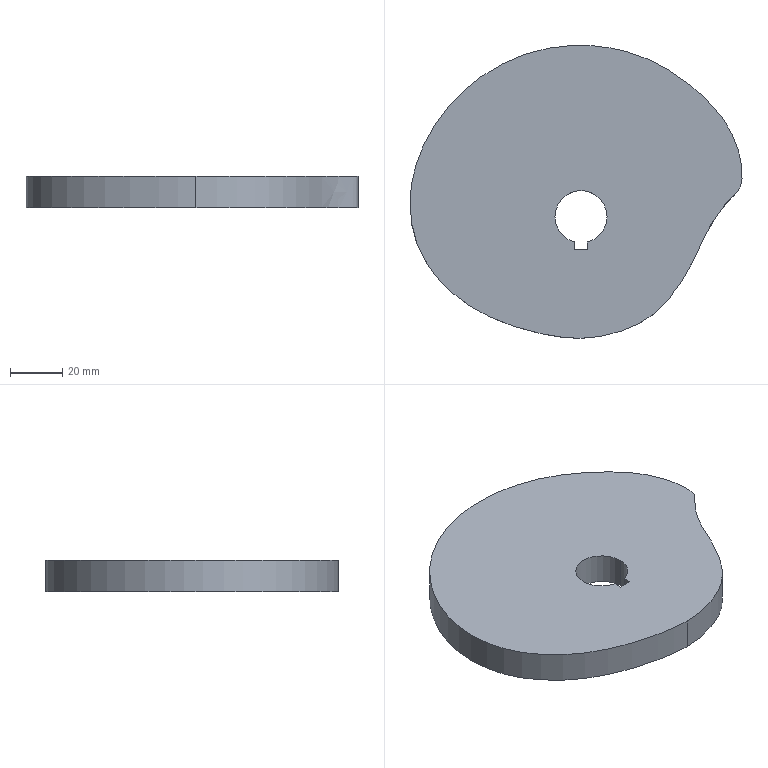Part | SolidWorks | features Extrusion 1 | 1 solid | 10 faces | box 127.495 x 112.48 x 12 mm | volume 126053 mm3 | plane 5 | cylinder 3 | spline 2 | commonest cylinder face diameters 20 x3
STEP:
#1=CARTESIAN_POINT('',(104.838,4.832,12.));
#2=VERTEX_POINT('',#1);
#3=CARTESIAN_POINT('',(99.807,-107.454,12.));
#4=VERTEX_POINT('',#3);
#5=CARTESIAN_POINT('',(104.838,4.832,12.));
#6=CARTESIAN_POINT('',(100.163,5.182,12.));
#7=CARTESIAN_POINT('',(90.7,4.929,12.));
#8=CARTESIAN_POINT('',(77.361,1.638,12.));
#9=CARTESIAN_POINT('',(64.795,-4.533,12.));
#10=CARTESIAN_POINT('',(55.618,-11.622,12.));
#11=CARTESIAN_POINT('',(49.26,-18.351,12.));
#12=CARTESIAN_POINT('',(43.576,-25.792,12.));
#13=CARTESIAN_POINT('',(39.125,-34.043,12.));
#14=CARTESIAN_POINT('',(36.234,-42.572,12.));
#15=CARTESIAN_POINT('',(34.893,-48.983,12.));
#16=CARTESIAN_POINT('',(34.421,-55.273,12.));
#17=CARTESIAN_POINT('',(34.796,-61.595,12.));
#18=CARTESIAN_POINT('',(35.964,-67.585,12.));
#19=CARTESIAN_POINT('',(37.777,-72.838,12.));
#20=CARTESIAN_POINT('',(40.255,-77.705,12.));
#21=CARTESIAN_POINT('',(43.305,-82.213,12.));
#22=CARTESIAN_POINT('',(46.799,-86.338,12.));
#23=CARTESIAN_POINT('',(51.787,-91.146,12.));
#24=CARTESIAN_POINT('',(58.741,-96.133,12.));
#25=CARTESIAN_POINT('',(66.65,-100.026,12.));
#26=CARTESIAN_POINT('',(73.439,-102.579,12.));
#27=CARTESIAN_POINT('',(78.673,-104.2,12.));
#28=CARTESIAN_POINT('',(84.12,-105.561,12.));
#29=CARTESIAN_POINT('',(89.642,-106.65,12.));
#30=CARTESIAN_POINT('',(94.019,-107.214,12.));
#31=CARTESIAN_POINT('',(97.386,-107.433,12.));
#32=CARTESIAN_POINT('',(99.005,-107.461,12.));
#33=CARTESIAN_POINT('',(99.807,-107.454,12.));
#34=B_SPLINE_CURVE_WITH_KNOTS('',3,(#5,#6,#7,#8,#9,#10,#11,#12,#13,#14,#15,#16,#17,#18,#19,#20,#21,#22,#23,#24,#25,#26,#27,#28,#29,#30,#31,#32,#33),.UNSPECIFIED.,.F.,.F.,(4,1,1,1,1,1,1,1,1,1,1,1,1,1,1,1,1,1,1,1,1,1,1,1,1,1,4),(1.5,1.531,1.562,1.594,1.625,1.641,1.656,1.687,1.703,1.719,1.734,1.75,1.766,1.781,1.797,1.812,1.828,1.844,1.875,1.906,1.922,1.937,1.953,1.969,1.984,1.992,2.),.UNSPECIFIED.);
#35=EDGE_CURVE('',#2,#4,#34,.T.);
#36=ORIENTED_EDGE('',*,*,#35,.F.);
#37=CARTESIAN_POINT('',(104.838,4.832,0.));
#38=VERTEX_POINT('',#37);
#39=CARTESIAN_POINT('',(104.838,4.832,12.));
#40=DIRECTION('',(0.,0.,-1.));
#41=VECTOR('',#40,1000.);
#42=LINE('',#39,#41);
#43=EDGE_CURVE('',#2,#38,#42,.T.);
#44=ORIENTED_EDGE('',*,*,#43,.T.);
#45=CARTESIAN_POINT('',(99.807,-107.454,0.));
#46=VERTEX_POINT('',#45);
#47=CARTESIAN_POINT('',(104.838,4.832,0.));
#48=CARTESIAN_POINT('',(100.163,5.182,0.));
#49=CARTESIAN_POINT('',(90.7,4.929,0.));
#50=CARTESIAN_POINT('',(77.361,1.638,0.));
#51=CARTESIAN_POINT('',(64.795,-4.533,0.));
#52=CARTESIAN_POINT('',(55.618,-11.622,0.));
#53=CARTESIAN_POINT('',(49.26,-18.351,0.));
#54=CARTESIAN_POINT('',(43.576,-25.792,0.));
#55=CARTESIAN_POINT('',(39.125,-34.043,0.));
#56=CARTESIAN_POINT('',(36.234,-42.572,0.));
#57=CARTESIAN_POINT('',(34.893,-48.983,0.));
#58=CARTESIAN_POINT('',(34.421,-55.273,0.));
#59=CARTESIAN_POINT('',(34.796,-61.595,0.));
#60=CARTESIAN_POINT('',(35.964,-67.585,0.));
#61=CARTESIAN_POINT('',(37.777,-72.838,0.));
#62=CARTESIAN_POINT('',(40.255,-77.705,0.));
#63=CARTESIAN_POINT('',(43.305,-82.213,0.));
#64=CARTESIAN_POINT('',(46.799,-86.338,0.));
#65=CARTESIAN_POINT('',(51.787,-91.146,0.));
#66=CARTESIAN_POINT('',(58.741,-96.133,0.));
#67=CARTESIAN_POINT('',(66.65,-100.026,0.));
#68=CARTESIAN_POINT('',(73.439,-102.579,0.));
#69=CARTESIAN_POINT('',(78.673,-104.2,0.));
#70=CARTESIAN_POINT('',(84.12,-105.561,0.));
#71=CARTESIAN_POINT('',(89.642,-106.65,0.));
#72=CARTESIAN_POINT('',(94.019,-107.214,0.));
#73=CARTESIAN_POINT('',(97.386,-107.433,0.));
#74=CARTESIAN_POINT('',(99.005,-107.461,0.));
#75=CARTESIAN_POINT('',(99.807,-107.454,0.));
#76=B_SPLINE_CURVE_WITH_KNOTS('',3,(#47,#48,#49,#50,#51,#52,#53,#54,#55,#56,#57,#58,#59,#60,#61,#62,#63,#64,#65,#66,#67,#68,#69,#70,#71,#72,#73,#74,#75),.UNSPECIFIED.,.F.,.F.,(4,1,1,1,1,1,1,1,1,1,1,1,1,1,1,1,1,1,1,1,1,1,1,1,1,1,4),(1.5,1.531,1.562,1.594,1.625,1.641,1.656,1.687,1.703,1.719,1.734,1.75,1.766,1.781,1.797,1.812,1.828,1.844,1.875,1.906,1.922,1.937,1.953,1.969,1.984,1.992,2.),.UNSPECIFIED.);
#77=EDGE_CURVE('',#38,#46,#76,.T.);
#78=ORIENTED_EDGE('',*,*,#77,.T.);
#79=CARTESIAN_POINT('',(99.807,-107.454,12.));
#80=DIRECTION('',(0.,0.,-1.));
#81=VECTOR('',#80,1000.);
#82=LINE('',#79,#81);
#83=EDGE_CURVE('',#4,#46,#82,.T.);
#84=ORIENTED_EDGE('',*,*,#83,.F.);
#85=EDGE_LOOP('',(#36,#44,#78,#84));
#86=FACE_OUTER_BOUND('',#85,.T.);
#87=CARTESIAN_POINT('',(104.838,4.832,12.));
#88=CARTESIAN_POINT('',(104.838,4.832,0.));
#89=CARTESIAN_POINT('',(100.163,5.182,12.));
#90=CARTESIAN_POINT('',(100.163,5.182,0.));
#91=CARTESIAN_POINT('',(90.7,4.929,12.));
#92=CARTESIAN_POINT('',(90.7,4.929,0.));
#93=CARTESIAN_POINT('',(77.361,1.638,12.));
#94=CARTESIAN_POINT('',(77.361,1.638,0.));
#95=CARTESIAN_POINT('',(64.795,-4.533,12.));
#96=CARTESIAN_POINT('',(64.795,-4.533,0.));
#97=CARTESIAN_POINT('',(55.618,-11.622,12.));
#98=CARTESIAN_POINT('',(55.618,-11.622,0.));
#99=CARTESIAN_POINT('',(49.26,-18.351,12.));
#100=CARTESIAN_POINT('',(49.26,-18.351,0.));
#101=CARTESIAN_POINT('',(43.576,-25.792,12.));
#102=CARTESIAN_POINT('',(43.576,-25.792,0.));
#103=CARTESIAN_POINT('',(39.125,-34.043,12.));
#104=CARTESIAN_POINT('',(39.125,-34.043,0.));
#105=CARTESIAN_POINT('',(36.234,-42.572,12.));
#106=CARTESIAN_POINT('',(36.234,-42.572,0.));
#107=CARTESIAN_POINT('',(34.893,-48.983,12.));
#108=CARTESIAN_POINT('',(34.893,-48.983,0.));
#109=CARTESIAN_POINT('',(34.421,-55.273,12.));
#110=CARTESIAN_POINT('',(34.421,-55.273,0.));
#111=CARTESIAN_POINT('',(34.796,-61.595,12.));
#112=CARTESIAN_POINT('',(34.796,-61.595,0.));
#113=CARTESIAN_POINT('',(35.964,-67.585,12.));
#114=CARTESIAN_POINT('',(35.964,-67.585,0.));
#115=CARTESIAN_POINT('',(37.777,-72.838,12.));
#116=CARTESIAN_POINT('',(37.777,-72.838,0.));
#117=CARTESIAN_POINT('',(40.255,-77.705,12.));
#118=CARTESIAN_POINT('',(40.255,-77.705,0.));
#119=CARTESIAN_POINT('',(43.305,-82.213,12.));
#120=CARTESIAN_POINT('',(43.305,-82.213,0.));
#121=CARTESIAN_POINT('',(46.799,-86.338,12.));
#122=CARTESIAN_POINT('',(46.799,-86.338,0.));
#123=CARTESIAN_POINT('',(51.787,-91.146,12.));
#124=CARTESIAN_POINT('',(51.787,-91.146,0.));
#125=CARTESIAN_POINT('',(58.741,-96.133,12.));
#126=CARTESIAN_POINT('',(58.741,-96.133,0.));
#127=CARTESIAN_POINT('',(66.65,-100.026,12.));
#128=CARTESIAN_POINT('',(66.65,-100.026,0.));
#129=CARTESIAN_POINT('',(73.439,-102.579,12.));
#130=CARTESIAN_POINT('',(73.439,-102.579,0.));
#131=CARTESIAN_POINT('',(78.673,-104.2,12.));
#132=CARTESIAN_POINT('',(78.673,-104.2,0.));
#133=CARTESIAN_POINT('',(84.12,-105.561,12.));
#134=CARTESIAN_POINT('',(84.12,-105.561,0.));
#135=CARTESIAN_POINT('',(89.642,-106.65,12.));
#136=CARTESIAN_POINT('',(89.642,-106.65,0.));
#137=CARTESIAN_POINT('',(94.019,-107.214,12.));
#138=CARTESIAN_POINT('',(94.019,-107.214,0.));
#139=CARTESIAN_POINT('',(97.386,-107.433,12.));
#140=CARTESIAN_POINT('',(97.386,-107.433,0.));
#141=CARTESIAN_POINT('',(99.005,-107.461,12.));
#142=CARTESIAN_POINT('',(99.005,-107.461,0.));
#143=CARTESIAN_POINT('',(99.807,-107.454,12.));
#144=CARTESIAN_POINT('',(99.807,-107.454,0.));
#145=B_SPLINE_SURFACE_WITH_KNOTS('',3,1,((#87,#88),(#89,#90),(#91,#92),(#93,#94),(#95,#96),(#97,#98),(#99,#100),(#101,#102),(#103,#104),(#105,#106),(#107,#108),(#109,#110),(#111,#112),(#113,#114),(#115,#116),(#117,#118),(#119,#120),(#121,#122),(#123,#124),(#125,#126),(#127,#128),(#129,#130),(#131,#132),(#133,#134),(#135,#136),(#137,#138),(#139,#140),(#141,#142),(#143,#144)),.UNSPECIFIED.,.F.,.F.,.F.,(4,1,1,1,1,1,1,1,1,1,1,1,1,1,1,1,1,1,1,1,1,1,1,1,1,1,4),(2,2),(1.5,1.531,1.562,1.594,1.625,1.641,1.656,1.687,1.703,1.719,1.734,1.75,1.766,1.781,1.797,1.812,1.828,1.844,1.875,1.906,1.922,1.937,1.953,1.969,1.984,1.992,2.),(0.,1.),.UNSPECIFIED.);
#146=ADVANCED_FACE('',(#86),#145,.F.);
#147=CARTESIAN_POINT('',(102.69,-70.461,12.));
#148=VERTEX_POINT('',#147);
#149=CARTESIAN_POINT('',(110.19,-60.778,12.));
#150=VERTEX_POINT('',#149);
#151=CARTESIAN_POINT('',(100.19,-60.778,12.));
#152=DIRECTION('',(0.,0.,1.));
#153=DIRECTION('',(1.,0.,0.));
#154=AXIS2_PLACEMENT_3D('',#151,#152,#153);
#155=CIRCLE('',#154,10.);
#156=EDGE_CURVE('',#148,#150,#155,.T.);
#157=ORIENTED_EDGE('',*,*,#156,.T.);
#158=CARTESIAN_POINT('',(110.19,-60.778,0.));
#159=VERTEX_POINT('',#158);
#160=CARTESIAN_POINT('',(110.19,-60.778,12.));
#161=DIRECTION('',(0.,0.,-1.));
#162=VECTOR('',#161,1000.);
#163=LINE('',#160,#162);
#164=EDGE_CURVE('',#150,#159,#163,.T.);
#165=ORIENTED_EDGE('',*,*,#164,.T.);
#166=CARTESIAN_POINT('',(102.69,-70.461,0.));
#167=VERTEX_POINT('',#166);
#168=CARTESIAN_POINT('',(100.19,-60.778,0.));
#169=DIRECTION('',(0.,0.,1.));
#170=DIRECTION('',(1.,0.,0.));
#171=AXIS2_PLACEMENT_3D('',#168,#169,#170);
#172=CIRCLE('',#171,10.);
#173=EDGE_CURVE('',#167,#159,#172,.T.);
#174=ORIENTED_EDGE('',*,*,#173,.F.);
#175=CARTESIAN_POINT('',(102.69,-70.461,12.));
#176=DIRECTION('',(0.,0.,-1.));
#177=VECTOR('',#176,1000.);
#178=LINE('',#175,#177);
#179=EDGE_CURVE('',#148,#167,#178,.T.);
#180=ORIENTED_EDGE('',*,*,#179,.F.);
#181=EDGE_LOOP('',(#157,#165,#174,#180));
#182=FACE_OUTER_BOUND('',#181,.T.);
#183=CARTESIAN_POINT('',(100.19,-60.778,12.));
#184=DIRECTION('',(0.,0.,-1.));
#185=DIRECTION('',(-1.,0.,0.));
#186=AXIS2_PLACEMENT_3D('',#183,#184,#185);
#187=CYLINDRICAL_SURFACE('',#186,10.);
#188=ADVANCED_FACE('',(#182),#187,.F.);
#189=ORIENTED_EDGE('',*,*,#164,.F.);
#190=CARTESIAN_POINT('',(90.19,-60.778,12.));
#191=VERTEX_POINT('',#190);
#192=CARTESIAN_POINT('',(100.19,-60.778,12.));
#193=DIRECTION('',(0.,0.,1.));
#194=DIRECTION('',(1.,0.,0.));
#195=AXIS2_PLACEMENT_3D('',#192,#193,#194);
#196=CIRCLE('',#195,10.);
#197=EDGE_CURVE('',#150,#191,#196,.T.);
#198=ORIENTED_EDGE('',*,*,#197,.T.);
#199=CARTESIAN_POINT('',(90.19,-60.778,0.));
#200=VERTEX_POINT('',#199);
#201=CARTESIAN_POINT('',(90.19,-60.778,12.));
#202=DIRECTION('',(0.,0.,-1.));
#203=VECTOR('',#202,1000.);
#204=LINE('',#201,#203);
#205=EDGE_CURVE('',#191,#200,#204,.T.);
#206=ORIENTED_EDGE('',*,*,#205,.T.);
#207=CARTESIAN_POINT('',(100.19,-60.778,0.));
#208=DIRECTION('',(0.,0.,1.));
#209=DIRECTION('',(1.,0.,0.));
#210=AXIS2_PLACEMENT_3D('',#207,#208,#209);
#211=CIRCLE('',#210,10.);
#212=EDGE_CURVE('',#159,#200,#211,.T.);
#213=ORIENTED_EDGE('',*,*,#212,.F.);
#214=EDGE_LOOP('',(#189,#198,#206,#213));
#215=FACE_OUTER_BOUND('',#214,.T.);
#216=CARTESIAN_POINT('',(100.19,-60.778,12.));
#217=DIRECTION('',(0.,0.,-1.));
#218=DIRECTION('',(-1.,0.,0.));
#219=AXIS2_PLACEMENT_3D('',#216,#217,#218);
#220=CYLINDRICAL_SURFACE('',#219,10.);
#221=ADVANCED_FACE('',(#215),#220,.F.);
#222=ORIENTED_EDGE('',*,*,#205,.F.);
#223=CARTESIAN_POINT('',(97.69,-70.461,12.));
#224=VERTEX_POINT('',#223);
#225=CARTESIAN_POINT('',(100.19,-60.778,12.));
#226=DIRECTION('',(0.,0.,1.));
#227=DIRECTION('',(1.,0.,0.));
#228=AXIS2_PLACEMENT_3D('',#225,#226,#227);
#229=CIRCLE('',#228,10.);
#230=EDGE_CURVE('',#191,#224,#229,.T.);
#231=ORIENTED_EDGE('',*,*,#230,.T.);
#232=CARTESIAN_POINT('',(97.69,-70.461,0.));
#233=VERTEX_POINT('',#232);
#234=CARTESIAN_POINT('',(97.69,-70.461,12.));
#235=DIRECTION('',(0.,0.,-1.));
#236=VECTOR('',#235,1000.);
#237=LINE('',#234,#236);
#238=EDGE_CURVE('',#224,#233,#237,.T.);
#239=ORIENTED_EDGE('',*,*,#238,.T.);
#240=CARTESIAN_POINT('',(100.19,-60.778,0.));
#241=DIRECTION('',(0.,0.,1.));
#242=DIRECTION('',(1.,0.,0.));
#243=AXIS2_PLACEMENT_3D('',#240,#241,#242);
#244=CIRCLE('',#243,10.);
#245=EDGE_CURVE('',#200,#233,#244,.T.);
#246=ORIENTED_EDGE('',*,*,#245,.F.);
#247=EDGE_LOOP('',(#222,#231,#239,#246));
#248=FACE_OUTER_BOUND('',#247,.T.);
#249=CARTESIAN_POINT('',(100.19,-60.778,12.));
#250=DIRECTION('',(0.,0.,-1.));
#251=DIRECTION('',(-1.,0.,0.));
#252=AXIS2_PLACEMENT_3D('',#249,#250,#251);
#253=CYLINDRICAL_SURFACE('',#252,10.);
#254=ADVANCED_FACE('',(#248),#253,.F.);
#255=CARTESIAN_POINT('',(102.69,-73.461,0.));
#256=VERTEX_POINT('',#255);
#257=CARTESIAN_POINT('',(102.69,0.,0.));
#258=DIRECTION('',(0.,1.,0.));
#259=VECTOR('',#258,1000.);
#260=LINE('',#257,#259);
#261=EDGE_CURVE('',#256,#167,#260,.T.);
#262=ORIENTED_EDGE('',*,*,#261,.F.);
#263=CARTESIAN_POINT('',(102.69,-73.461,12.));
#264=VERTEX_POINT('',#263);
#265=CARTESIAN_POINT('',(102.69,-73.461,12.));
#266=DIRECTION('',(0.,0.,-1.));
#267=VECTOR('',#266,1000.);
#268=LINE('',#265,#267);
#269=EDGE_CURVE('',#264,#256,#268,.T.);
#270=ORIENTED_EDGE('',*,*,#269,.F.);
#271=CARTESIAN_POINT('',(102.69,0.,12.));
#272=DIRECTION('',(0.,1.,0.));
#273=VECTOR('',#272,1000.);
#274=LINE('',#271,#273);
#275=EDGE_CURVE('',#264,#148,#274,.T.);
#276=ORIENTED_EDGE('',*,*,#275,.T.);
#277=ORIENTED_EDGE('',*,*,#179,.T.);
#278=EDGE_LOOP('',(#262,#270,#276,#277));
#279=FACE_OUTER_BOUND('',#278,.T.);
#280=CARTESIAN_POINT('',(102.69,0.,12.));
#281=DIRECTION('',(-1.,0.,0.));
#282=DIRECTION('',(0.,0.,1.));
#283=AXIS2_PLACEMENT_3D('',#280,#281,#282);
#284=PLANE('',#283);
#285=ADVANCED_FACE('',(#279),#284,.T.);
#286=CARTESIAN_POINT('',(97.69,-73.461,0.));
#287=VERTEX_POINT('',#286);
#288=CARTESIAN_POINT('',(0.,-73.461,0.));
#289=DIRECTION('',(1.,0.,0.));
#290=VECTOR('',#289,1000.);
#291=LINE('',#288,#290);
#292=EDGE_CURVE('',#287,#256,#291,.T.);
#293=ORIENTED_EDGE('',*,*,#292,.F.);
#294=CARTESIAN_POINT('',(97.69,-73.461,12.));
#295=VERTEX_POINT('',#294);
#296=CARTESIAN_POINT('',(97.69,-73.461,12.));
#297=DIRECTION('',(0.,0.,-1.));
#298=VECTOR('',#297,1000.);
#299=LINE('',#296,#298);
#300=EDGE_CURVE('',#295,#287,#299,.T.);
#301=ORIENTED_EDGE('',*,*,#300,.F.);
#302=CARTESIAN_POINT('',(0.,-73.461,12.));
#303=DIRECTION('',(1.,0.,0.));
#304=VECTOR('',#303,1000.);
#305=LINE('',#302,#304);
#306=EDGE_CURVE('',#295,#264,#305,.T.);
#307=ORIENTED_EDGE('',*,*,#306,.T.);
#308=ORIENTED_EDGE('',*,*,#269,.T.);
#309=EDGE_LOOP('',(#293,#301,#307,#308));
#310=FACE_OUTER_BOUND('',#309,.T.);
#311=CARTESIAN_POINT('',(0.,-73.461,12.));
#312=DIRECTION('',(0.,1.,0.));
#313=DIRECTION('',(0.,0.,1.));
#314=AXIS2_PLACEMENT_3D('',#311,#312,#313);
#315=PLANE('',#314);
#316=ADVANCED_FACE('',(#310),#315,.T.);
#317=CARTESIAN_POINT('',(97.69,0.,0.));
#318=DIRECTION('',(0.,-1.,0.));
#319=VECTOR('',#318,1000.);
#320=LINE('',#317,#319);
#321=EDGE_CURVE('',#233,#287,#320,.T.);
#322=ORIENTED_EDGE('',*,*,#321,.F.);
#323=ORIENTED_EDGE('',*,*,#238,.F.);
#324=CARTESIAN_POINT('',(97.69,0.,12.));
#325=DIRECTION('',(0.,-1.,0.));
#326=VECTOR('',#325,1000.);
#327=LINE('',#324,#326);
#328=EDGE_CURVE('',#224,#295,#327,.T.);
#329=ORIENTED_EDGE('',*,*,#328,.T.);
#330=ORIENTED_EDGE('',*,*,#300,.T.);
#331=EDGE_LOOP('',(#322,#323,#329,#330));
#332=FACE_OUTER_BOUND('',#331,.T.);
#333=CARTESIAN_POINT('',(97.69,0.,12.));
#334=DIRECTION('',(1.,0.,0.));
#335=DIRECTION('',(0.,0.,-1.));
#336=AXIS2_PLACEMENT_3D('',#333,#334,#335);
#337=PLANE('',#336);
#338=ADVANCED_FACE('',(#332),#337,.T.);
#339=ORIENTED_EDGE('',*,*,#43,.F.);
#340=CARTESIAN_POINT('',(99.807,-107.454,12.));
#341=CARTESIAN_POINT('',(100.61,-107.446,12.));
#342=CARTESIAN_POINT('',(102.201,-107.389,12.));
#343=CARTESIAN_POINT('',(105.417,-107.107,12.));
#344=CARTESIAN_POINT('',(109.447,-106.446,12.));
#345=CARTESIAN_POINT('',(114.36,-105.152,12.));
#346=CARTESIAN_POINT('',(119.109,-103.43,12.));
#347=CARTESIAN_POINT('',(122.698,-101.687,12.));
#348=CARTESIAN_POINT('',(125.31,-100.119,12.));
#349=CARTESIAN_POINT('',(127.702,-98.464,12.));
#350=CARTESIAN_POINT('',(130.598,-96.011,12.));
#351=CARTESIAN_POINT('',(133.917,-92.475,12.));
#352=CARTESIAN_POINT('',(137.044,-88.421,12.));
#353=CARTESIAN_POINT('',(139.944,-83.955,12.));
#354=CARTESIAN_POINT('',(142.155,-79.986,12.));
#355=CARTESIAN_POINT('',(143.791,-76.739,12.));
#356=CARTESIAN_POINT('',(145.353,-73.427,12.));
#357=CARTESIAN_POINT('',(147.04,-69.661,12.));
#358=CARTESIAN_POINT('',(149.057,-65.59,12.));
#359=CARTESIAN_POINT('',(150.546,-62.921,12.));
#360=CARTESIAN_POINT('',(151.933,-60.734,12.));
#361=CARTESIAN_POINT('',(153.102,-59.062,12.));
#362=CARTESIAN_POINT('',(154.38,-57.427,12.));
#363=CARTESIAN_POINT('',(155.986,-55.56,12.));
#364=CARTESIAN_POINT('',(157.802,-53.658,12.));
#365=CARTESIAN_POINT('',(159.462,-51.974,12.));
#366=CARTESIAN_POINT('',(160.538,-50.795,12.));
#367=CARTESIAN_POINT('',(160.977,-50.212,12.));
#368=CARTESIAN_POINT('',(161.157,-49.925,12.));
#369=CARTESIAN_POINT('',(161.223,-49.803,12.));
#370=CARTESIAN_POINT('',(161.324,-49.582,12.));
#371=CARTESIAN_POINT('',(161.505,-49.096,12.));
#372=CARTESIAN_POINT('',(161.757,-48.166,12.));
#373=CARTESIAN_POINT('',(162.071,-46.065,12.));
#374=CARTESIAN_POINT('',(162.107,-42.495,12.));
#375=CARTESIAN_POINT('',(161.288,-37.303,12.));
#376=CARTESIAN_POINT('',(159.529,-31.714,12.));
#377=CARTESIAN_POINT('',(157.272,-27.067,12.));
#378=CARTESIAN_POINT('',(155.036,-23.563,12.));
#379=CARTESIAN_POINT('',(152.371,-20.001,12.));
#380=CARTESIAN_POINT('',(148.342,-15.573,12.));
#381=CARTESIAN_POINT('',(143.67,-11.409,12.));
#382=CARTESIAN_POINT('',(139.764,-8.354,12.));
#383=CARTESIAN_POINT('',(135.88,-5.581,12.));
#384=CARTESIAN_POINT('',(130.987,-2.593,12.));
#385=CARTESIAN_POINT('',(124.973,0.2716,12.));
#386=CARTESIAN_POINT('',(118.584,2.493,12.));
#387=CARTESIAN_POINT('',(111.821,4.068,12.));
#388=CARTESIAN_POINT('',(107.175,4.656,12.));
#389=CARTESIAN_POINT('',(104.838,4.832,12.));
#390=B_SPLINE_CURVE_WITH_KNOTS('',3,(#340,#341,#342,#343,#344,#345,#346,#347,#348,#349,#350,#351,#352,#353,#354,#355,#356,#357,#358,#359,#360,#361,#362,#363,#364,#365,#366,#367,#368,#369,#370,#371,#372,#373,#374,#375,#376,#377,#378,#379,#380,#381,#382,#383,#384,#385,#386,#387,#388,#389),.UNSPECIFIED.,.F.,.F.,(4,1,1,1,1,1,1,1,1,1,1,1,1,1,1,1,1,1,1,1,1,1,1,1,1,1,1,1,1,1,1,1,1,1,1,1,1,1,1,1,1,1,1,1,1,1,1,4),(1.,1.008,1.016,1.031,1.047,1.062,1.078,1.086,1.094,1.109,1.125,1.141,1.156,1.172,1.18,1.187,1.203,1.211,1.219,1.223,1.227,1.23,1.234,1.242,1.25,1.258,1.266,1.27,1.273,1.277,1.281,1.289,1.297,1.312,1.328,1.344,1.359,1.367,1.375,1.391,1.406,1.414,1.422,1.437,1.453,1.469,1.484,1.5),.UNSPECIFIED.);
#391=EDGE_CURVE('',#4,#2,#390,.T.);
#392=ORIENTED_EDGE('',*,*,#391,.F.);
#393=ORIENTED_EDGE('',*,*,#83,.T.);
#394=CARTESIAN_POINT('',(99.807,-107.454,0.));
#395=CARTESIAN_POINT('',(100.61,-107.446,0.));
#396=CARTESIAN_POINT('',(102.201,-107.389,0.));
#397=CARTESIAN_POINT('',(105.417,-107.107,0.));
#398=CARTESIAN_POINT('',(109.447,-106.446,0.));
#399=CARTESIAN_POINT('',(114.36,-105.152,0.));
#400=CARTESIAN_POINT('',(119.109,-103.43,0.));
#401=CARTESIAN_POINT('',(122.698,-101.687,0.));
#402=CARTESIAN_POINT('',(125.31,-100.119,0.));
#403=CARTESIAN_POINT('',(127.702,-98.464,0.));
#404=CARTESIAN_POINT('',(130.598,-96.011,0.));
#405=CARTESIAN_POINT('',(133.917,-92.475,0.));
#406=CARTESIAN_POINT('',(137.044,-88.421,0.));
#407=CARTESIAN_POINT('',(139.944,-83.955,0.));
#408=CARTESIAN_POINT('',(142.155,-79.986,0.));
#409=CARTESIAN_POINT('',(143.791,-76.739,0.));
#410=CARTESIAN_POINT('',(145.353,-73.427,0.));
#411=CARTESIAN_POINT('',(147.04,-69.661,0.));
#412=CARTESIAN_POINT('',(149.057,-65.59,0.));
#413=CARTESIAN_POINT('',(150.546,-62.921,0.));
#414=CARTESIAN_POINT('',(151.933,-60.734,0.));
#415=CARTESIAN_POINT('',(153.102,-59.062,0.));
#416=CARTESIAN_POINT('',(154.38,-57.427,0.));
#417=CARTESIAN_POINT('',(155.986,-55.56,0.));
#418=CARTESIAN_POINT('',(157.802,-53.658,0.));
#419=CARTESIAN_POINT('',(159.462,-51.974,0.));
#420=CARTESIAN_POINT('',(160.538,-50.795,0.));
#421=CARTESIAN_POINT('',(160.977,-50.212,0.));
#422=CARTESIAN_POINT('',(161.157,-49.925,0.));
#423=CARTESIAN_POINT('',(161.223,-49.803,0.));
#424=CARTESIAN_POINT('',(161.324,-49.582,0.));
#425=CARTESIAN_POINT('',(161.505,-49.096,0.));
#426=CARTESIAN_POINT('',(161.757,-48.166,0.));
#427=CARTESIAN_POINT('',(162.071,-46.065,0.));
#428=CARTESIAN_POINT('',(162.107,-42.495,0.));
#429=CARTESIAN_POINT('',(161.288,-37.303,0.));
#430=CARTESIAN_POINT('',(159.529,-31.714,0.));
#431=CARTESIAN_POINT('',(157.272,-27.067,0.));
#432=CARTESIAN_POINT('',(155.036,-23.563,0.));
#433=CARTESIAN_POINT('',(152.371,-20.001,0.));
#434=CARTESIAN_POINT('',(148.342,-15.573,0.));
#435=CARTESIAN_POINT('',(143.67,-11.409,0.));
#436=CARTESIAN_POINT('',(139.764,-8.354,0.));
#437=CARTESIAN_POINT('',(135.88,-5.581,0.));
#438=CARTESIAN_POINT('',(130.987,-2.593,0.));
#439=CARTESIAN_POINT('',(124.973,0.2716,0.));
#440=CARTESIAN_POINT('',(118.584,2.493,0.));
#441=CARTESIAN_POINT('',(111.821,4.068,0.));
#442=CARTESIAN_POINT('',(107.175,4.656,0.));
#443=CARTESIAN_POINT('',(104.838,4.832,0.));
#444=B_SPLINE_CURVE_WITH_KNOTS('',3,(#394,#395,#396,#397,#398,#399,#400,#401,#402,#403,#404,#405,#406,#407,#408,#409,#410,#411,#412,#413,#414,#415,#416,#417,#418,#419,#420,#421,#422,#423,#424,#425,#426,#427,#428,#429,#430,#431,#432,#433,#434,#435,#436,#437,#438,#439,#440,#441,#442,#443),.UNSPECIFIED.,.F.,.F.,(4,1,1,1,1,1,1,1,1,1,1,1,1,1,1,1,1,1,1,1,1,1,1,1,1,1,1,1,1,1,1,1,1,1,1,1,1,1,1,1,1,1,1,1,1,1,1,4),(1.,1.008,1.016,1.031,1.047,1.062,1.078,1.086,1.094,1.109,1.125,1.141,1.156,1.172,1.18,1.187,1.203,1.211,1.219,1.223,1.227,1.23,1.234,1.242,1.25,1.258,1.266,1.27,1.273,1.277,1.281,1.289,1.297,1.312,1.328,1.344,1.359,1.367,1.375,1.391,1.406,1.414,1.422,1.437,1.453,1.469,1.484,1.5),.UNSPECIFIED.);
#445=EDGE_CURVE('',#46,#38,#444,.T.);
#446=ORIENTED_EDGE('',*,*,#445,.T.);
#447=EDGE_LOOP('',(#339,#392,#393,#446));
#448=FACE_OUTER_BOUND('',#447,.T.);
#449=CARTESIAN_POINT('',(99.807,-107.454,12.));
#450=CARTESIAN_POINT('',(99.807,-107.454,0.));
#451=CARTESIAN_POINT('',(100.61,-107.446,12.));
#452=CARTESIAN_POINT('',(100.61,-107.446,0.));
#453=CARTESIAN_POINT('',(102.201,-107.389,12.));
#454=CARTESIAN_POINT('',(102.201,-107.389,0.));
#455=CARTESIAN_POINT('',(105.417,-107.107,12.));
#456=CARTESIAN_POINT('',(105.417,-107.107,0.));
#457=CARTESIAN_POINT('',(109.447,-106.446,12.));
#458=CARTESIAN_POINT('',(109.447,-106.446,0.));
#459=CARTESIAN_POINT('',(114.36,-105.152,12.));
#460=CARTESIAN_POINT('',(114.36,-105.152,0.));
#461=CARTESIAN_POINT('',(119.109,-103.43,12.));
#462=CARTESIAN_POINT('',(119.109,-103.43,0.));
#463=CARTESIAN_POINT('',(122.698,-101.687,12.));
#464=CARTESIAN_POINT('',(122.698,-101.687,0.));
#465=CARTESIAN_POINT('',(125.31,-100.119,12.));
#466=CARTESIAN_POINT('',(125.31,-100.119,0.));
#467=CARTESIAN_POINT('',(127.702,-98.464,12.));
#468=CARTESIAN_POINT('',(127.702,-98.464,0.));
#469=CARTESIAN_POINT('',(130.598,-96.011,12.));
#470=CARTESIAN_POINT('',(130.598,-96.011,0.));
#471=CARTESIAN_POINT('',(133.917,-92.475,12.));
#472=CARTESIAN_POINT('',(133.917,-92.475,0.));
#473=CARTESIAN_POINT('',(137.044,-88.421,12.));
#474=CARTESIAN_POINT('',(137.044,-88.421,0.));
#475=CARTESIAN_POINT('',(139.944,-83.955,12.));
#476=CARTESIAN_POINT('',(139.944,-83.955,0.));
#477=CARTESIAN_POINT('',(142.155,-79.986,12.));
#478=CARTESIAN_POINT('',(142.155,-79.986,0.));
#479=CARTESIAN_POINT('',(143.791,-76.739,12.));
#480=CARTESIAN_POINT('',(143.791,-76.739,0.));
#481=CARTESIAN_POINT('',(145.353,-73.427,12.));
#482=CARTESIAN_POINT('',(145.353,-73.427,0.));
#483=CARTESIAN_POINT('',(147.04,-69.661,12.));
#484=CARTESIAN_POINT('',(147.04,-69.661,0.));
#485=CARTESIAN_POINT('',(149.057,-65.59,12.));
#486=CARTESIAN_POINT('',(149.057,-65.59,0.));
#487=CARTESIAN_POINT('',(150.546,-62.921,12.));
#488=CARTESIAN_POINT('',(150.546,-62.921,0.));
#489=CARTESIAN_POINT('',(151.933,-60.734,12.));
#490=CARTESIAN_POINT('',(151.933,-60.734,0.));
#491=CARTESIAN_POINT('',(153.102,-59.062,12.));
#492=CARTESIAN_POINT('',(153.102,-59.062,0.));
#493=CARTESIAN_POINT('',(154.38,-57.427,12.));
#494=CARTESIAN_POINT('',(154.38,-57.427,0.));
#495=CARTESIAN_POINT('',(155.986,-55.56,12.));
#496=CARTESIAN_POINT('',(155.986,-55.56,0.));
#497=CARTESIAN_POINT('',(157.802,-53.658,12.));
#498=CARTESIAN_POINT('',(157.802,-53.658,0.));
#499=CARTESIAN_POINT('',(159.462,-51.974,12.));
#500=CARTESIAN_POINT('',(159.462,-51.974,0.));
#501=CARTESIAN_POINT('',(160.538,-50.795,12.));
#502=CARTESIAN_POINT('',(160.538,-50.795,0.));
#503=CARTESIAN_POINT('',(160.977,-50.212,12.));
#504=CARTESIAN_POINT('',(160.977,-50.212,0.));
#505=CARTESIAN_POINT('',(161.157,-49.925,12.));
#506=CARTESIAN_POINT('',(161.157,-49.925,0.));
#507=CARTESIAN_POINT('',(161.223,-49.803,12.));
#508=CARTESIAN_POINT('',(161.223,-49.803,0.));
#509=CARTESIAN_POINT('',(161.324,-49.582,12.));
#510=CARTESIAN_POINT('',(161.324,-49.582,0.));
#511=CARTESIAN_POINT('',(161.505,-49.096,12.));
#512=CARTESIAN_POINT('',(161.505,-49.096,0.));
#513=CARTESIAN_POINT('',(161.757,-48.166,12.));
#514=CARTESIAN_POINT('',(161.757,-48.166,0.));
#515=CARTESIAN_POINT('',(162.071,-46.065,12.));
#516=CARTESIAN_POINT('',(162.071,-46.065,0.));
#517=CARTESIAN_POINT('',(162.107,-42.495,12.));
#518=CARTESIAN_POINT('',(162.107,-42.495,0.));
#519=CARTESIAN_POINT('',(161.288,-37.303,12.));
#520=CARTESIAN_POINT('',(161.288,-37.303,0.));
#521=CARTESIAN_POINT('',(159.529,-31.714,12.));
#522=CARTESIAN_POINT('',(159.529,-31.714,0.));
#523=CARTESIAN_POINT('',(157.272,-27.067,12.));
#524=CARTESIAN_POINT('',(157.272,-27.067,0.));
#525=CARTESIAN_POINT('',(155.036,-23.563,12.));
#526=CARTESIAN_POINT('',(155.036,-23.563,0.));
#527=CARTESIAN_POINT('',(152.371,-20.001,12.));
#528=CARTESIAN_POINT('',(152.371,-20.001,0.));
#529=CARTESIAN_POINT('',(148.342,-15.573,12.));
#530=CARTESIAN_POINT('',(148.342,-15.573,0.));
#531=CARTESIAN_POINT('',(143.67,-11.409,12.));
#532=CARTESIAN_POINT('',(143.67,-11.409,0.));
#533=CARTESIAN_POINT('',(139.764,-8.354,12.));
#534=CARTESIAN_POINT('',(139.764,-8.354,0.));
#535=CARTESIAN_POINT('',(135.88,-5.581,12.));
#536=CARTESIAN_POINT('',(135.88,-5.581,0.));
#537=CARTESIAN_POINT('',(130.987,-2.593,12.));
#538=CARTESIAN_POINT('',(130.987,-2.593,0.));
#539=CARTESIAN_POINT('',(124.973,0.2716,12.));
#540=CARTESIAN_POINT('',(124.973,0.2716,0.));
#541=CARTESIAN_POINT('',(118.584,2.493,12.));
#542=CARTESIAN_POINT('',(118.584,2.493,0.));
#543=CARTESIAN_POINT('',(111.821,4.068,12.));
#544=CARTESIAN_POINT('',(111.821,4.068,0.));
#545=CARTESIAN_POINT('',(107.175,4.656,12.));
#546=CARTESIAN_POINT('',(107.175,4.656,0.));
#547=CARTESIAN_POINT('',(104.838,4.832,12.));
#548=CARTESIAN_POINT('',(104.838,4.832,0.));
#549=B_SPLINE_SURFACE_WITH_KNOTS('',3,1,((#449,#450),(#451,#452),(#453,#454),(#455,#456),(#457,#458),(#459,#460),(#461,#462),(#463,#464),(#465,#466),(#467,#468),(#469,#470),(#471,#472),(#473,#474),(#475,#476),(#477,#478),(#479,#480),(#481,#482),(#483,#484),(#485,#486),(#487,#488),(#489,#490),(#491,#492),(#493,#494),(#495,#496),(#497,#498),(#499,#500),(#501,#502),(#503,#504),(#505,#506),(#507,#508),(#509,#510),(#511,#512),(#513,#514),(#515,#516),(#517,#518),(#519,#520),(#521,#522),(#523,#524),(#525,#526),(#527,#528),(#529,#530),(#531,#532),(#533,#534),(#535,#536),(#537,#538),(#539,#540),(#541,#542),(#543,#544),(#545,#546),(#547,#548)),.UNSPECIFIED.,.F.,.F.,.F.,(4,1,1,1,1,1,1,1,1,1,1,1,1,1,1,1,1,1,1,1,1,1,1,1,1,1,1,1,1,1,1,1,1,1,1,1,1,1,1,1,1,1,1,1,1,1,1,4),(2,2),(1.,1.008,1.016,1.031,1.047,1.062,1.078,1.086,1.094,1.109,1.125,1.141,1.156,1.172,1.18,1.187,1.203,1.211,1.219,1.223,1.227,1.23,1.234,1.242,1.25,1.258,1.266,1.27,1.273,1.277,1.281,1.289,1.297,1.312,1.328,1.344,1.359,1.367,1.375,1.391,1.406,1.414,1.422,1.437,1.453,1.469,1.484,1.5),(0.,1.),.UNSPECIFIED.);
#550=ADVANCED_FACE('',(#448),#549,.F.);
#551=ORIENTED_EDGE('',*,*,#156,.F.);
#552=ORIENTED_EDGE('',*,*,#275,.F.);
#553=ORIENTED_EDGE('',*,*,#306,.F.);
#554=ORIENTED_EDGE('',*,*,#328,.F.);
#555=ORIENTED_EDGE('',*,*,#230,.F.);
#556=ORIENTED_EDGE('',*,*,#197,.F.);
#557=EDGE_LOOP('',(#551,#552,#553,#554,#555,#556));
#558=FACE_BOUND('',#557,.T.);
#559=ORIENTED_EDGE('',*,*,#391,.T.);
#560=ORIENTED_EDGE('',*,*,#35,.T.);
#561=EDGE_LOOP('',(#559,#560));
#562=FACE_OUTER_BOUND('',#561,.T.);
#563=CARTESIAN_POINT('',(0.,0.,12.));
#564=DIRECTION('',(0.,0.,1.));
#565=DIRECTION('',(1.,0.,0.));
#566=AXIS2_PLACEMENT_3D('',#563,#564,#565);
#567=PLANE('',#566);
#568=ADVANCED_FACE('',(#558,#562),#567,.T.);
#569=ORIENTED_EDGE('',*,*,#173,.T.);
#570=ORIENTED_EDGE('',*,*,#212,.T.);
#571=ORIENTED_EDGE('',*,*,#245,.T.);
#572=ORIENTED_EDGE('',*,*,#321,.T.);
#573=ORIENTED_EDGE('',*,*,#292,.T.);
#574=ORIENTED_EDGE('',*,*,#261,.T.);
#575=EDGE_LOOP('',(#569,#570,#571,#572,#573,#574));
#576=FACE_BOUND('',#575,.T.);
#577=ORIENTED_EDGE('',*,*,#445,.F.);
#578=ORIENTED_EDGE('',*,*,#77,.F.);
#579=EDGE_LOOP('',(#577,#578));
#580=FACE_OUTER_BOUND('',#579,.T.);
#581=CARTESIAN_POINT('',(0.,0.,0.));
#582=DIRECTION('',(0.,0.,1.));
#583=DIRECTION('',(1.,0.,0.));
#584=AXIS2_PLACEMENT_3D('',#581,#582,#583);
#585=PLANE('',#584);
#586=ADVANCED_FACE('',(#576,#580),#585,.F.);
#587=CLOSED_SHELL('',(#146,#188,#221,#254,#285,#316,#338,#550,#568,#586));
#588=MANIFOLD_SOLID_BREP('',#587);
#589=CARTESIAN_POINT('',(0.,0.,0.));
#590=DIRECTION('',(0.,0.,1.));
#591=DIRECTION('',(1.,0.,0.));
#592=AXIS2_PLACEMENT_3D('',#589,#590,#591);
#593=(LENGTH_UNIT()NAMED_UNIT(*)SI_UNIT(.MILLI.,.METRE.));
#594=UNCERTAINTY_MEASURE_WITH_UNIT(LENGTH_MEASURE(0.00001),#593,'','');
#595=(NAMED_UNIT(*)PLANE_ANGLE_UNIT()SI_UNIT($,.RADIAN.));
#596=(NAMED_UNIT(*)SI_UNIT($,.STERADIAN.)SOLID_ANGLE_UNIT());
#597=(GEOMETRIC_REPRESENTATION_CONTEXT(3)GLOBAL_UNCERTAINTY_ASSIGNED_CONTEXT((#594))GLOBAL_UNIT_ASSIGNED_CONTEXT((#593,#595,#596))REPRESENTATION_CONTEXT('',''));
#598=ADVANCED_BREP_SHAPE_REPRESENTATION('',(#588,#592),#597);